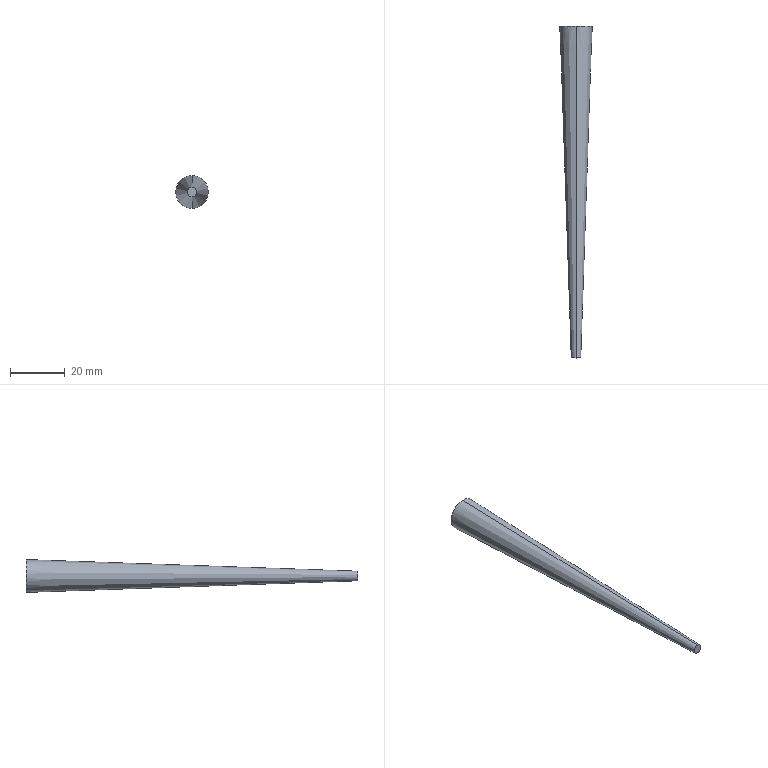Part | STEP file | 1 solid | 4 faces | box 12.021 x 121.757 x 12.021 mm | volume 6349 mm3 | cone 2 | plane 2
STEP:
#1=CARTESIAN_POINT('',(0.,0.,0.));
#2=DIRECTION('',(0.,0.,1.));
#3=DIRECTION('',(1.,0.,0.));
#4=AXIS2_PLACEMENT_3D('',#1,#2,#3);
#5=CARTESIAN_POINT('',(-137.183,8.743,9.799));
#6=VERTEX_POINT('',#5);
#7=CARTESIAN_POINT('',(-137.183,8.743,13.316));
#8=VERTEX_POINT('',#7);
#9=CARTESIAN_POINT('',(-137.183,8.743,11.557));
#10=DIRECTION('',(0.,1.,0.));
#11=DIRECTION('',(0.,0.,-1.));
#12=AXIS2_PLACEMENT_3D('',#9,#10,#11);
#13=CIRCLE('',#12,1.759);
#14=CARTESIAN_POINT('',(-137.183,8.743,11.557));
#15=DIRECTION('',(0.,1.,0.));
#16=DIRECTION('',(0.,0.,-1.));
#17=AXIS2_PLACEMENT_3D('',#14,#15,#16);
#18=CONICAL_SURFACE('',#17,1.759,0.03491);
#19=CARTESIAN_POINT('',(0.,0.));
#20=DIRECTION('',(1.,0.));
#21=VECTOR('',#20,1.);
#22=LINE('',#19,#21);
#23=(GEOMETRIC_REPRESENTATION_CONTEXT(2)PARAMETRIC_REPRESENTATION_CONTEXT()REPRESENTATION_CONTEXT('',''));
#24=DEFINITIONAL_REPRESENTATION('',(#22),#23);
#25=PCURVE('',#18,#24);
#26=CARTESIAN_POINT('',(-137.183,8.743,8.797));
#27=DIRECTION('',(0.,-1.,0.));
#28=DIRECTION('',(0.,0.,-1.));
#29=AXIS2_PLACEMENT_3D('',#26,#27,#28);
#30=PLANE('',#29);
#31=CARTESIAN_POINT('',(-1.001,0.));
#32=CARTESIAN_POINT('',(-1.001,-3.046));
#33=CARTESIAN_POINT('',(-3.64,-1.523));
#34=CARTESIAN_POINT('',(-6.278,0.));
#35=CARTESIAN_POINT('',(-3.64,1.523));
#36=CARTESIAN_POINT('',(-1.001,3.046));
#37=CARTESIAN_POINT('',(-1.001,0.));
#38=(BOUNDED_CURVE()B_SPLINE_CURVE(2,(#31,#32,#33,#34,#35,#36,#37),.UNSPECIFIED.,.T.,.F.)B_SPLINE_CURVE_WITH_KNOTS((1,2,2,2,2,1),(-2.094,0.,2.094,4.189,6.283,8.378),.UNSPECIFIED.)CURVE()GEOMETRIC_REPRESENTATION_ITEM()RATIONAL_B_SPLINE_CURVE((1.,0.5,1.,0.5,1.,0.5,1.))REPRESENTATION_ITEM(''));
#39=(GEOMETRIC_REPRESENTATION_CONTEXT(2)PARAMETRIC_REPRESENTATION_CONTEXT()REPRESENTATION_CONTEXT('',''));
#40=DEFINITIONAL_REPRESENTATION('',(#38),#39);
#41=PCURVE('',#30,#40);
#42=SURFACE_CURVE('',#13,(#25,#41),.PCURVE_S1.);
#43=EDGE_CURVE('',#6,#8,#42,.T.);
#44=ORIENTED_EDGE('',*,*,#43,.T.);
#45=CARTESIAN_POINT('',(-137.183,130.5,17.568));
#46=VERTEX_POINT('',#45);
#47=CARTESIAN_POINT('',(-137.183,8.743,13.316));
#48=DIRECTION('',(0.,0.9994,0.0349));
#49=VECTOR('',#48,1.);
#50=LINE('',#47,#49);
#51=CARTESIAN_POINT('',(3.142,0.));
#52=DIRECTION('',(0.,1.));
#53=VECTOR('',#52,1.);
#54=LINE('',#51,#53);
#55=(GEOMETRIC_REPRESENTATION_CONTEXT(2)PARAMETRIC_REPRESENTATION_CONTEXT()REPRESENTATION_CONTEXT('',''));
#56=DEFINITIONAL_REPRESENTATION('',(#54),#55);
#57=PCURVE('',#18,#56);
#58=CARTESIAN_POINT('',(-137.183,8.743,11.557));
#59=DIRECTION('',(0.,1.,0.));
#60=DIRECTION('',(0.,0.,-1.));
#61=AXIS2_PLACEMENT_3D('',#58,#59,#60);
#62=CONICAL_SURFACE('',#61,1.759,0.03491);
#63=CARTESIAN_POINT('',(3.142,0.));
#64=DIRECTION('',(0.,1.));
#65=VECTOR('',#64,1.);
#66=LINE('',#63,#65);
#67=(GEOMETRIC_REPRESENTATION_CONTEXT(2)PARAMETRIC_REPRESENTATION_CONTEXT()REPRESENTATION_CONTEXT('',''));
#68=DEFINITIONAL_REPRESENTATION('',(#66),#67);
#69=PCURVE('',#62,#68);
#70=SURFACE_CURVE('',#50,(#57,#69),.PCURVE_S1.);
#71=EDGE_CURVE('',#8,#46,#70,.T.);
#72=ORIENTED_EDGE('',*,*,#71,.T.);
#73=CARTESIAN_POINT('',(-137.183,130.5,5.547));
#74=VERTEX_POINT('',#73);
#75=CARTESIAN_POINT('',(-137.183,130.5,11.557));
#76=DIRECTION('',(0.,-1.,0.));
#77=DIRECTION('',(0.,0.,-1.));
#78=AXIS2_PLACEMENT_3D('',#75,#76,#77);
#79=CIRCLE('',#78,6.011);
#80=CARTESIAN_POINT('',(6.283,121.757));
#81=DIRECTION('',(-1.,0.));
#82=VECTOR('',#81,1.);
#83=LINE('',#80,#82);
#84=(GEOMETRIC_REPRESENTATION_CONTEXT(2)PARAMETRIC_REPRESENTATION_CONTEXT()REPRESENTATION_CONTEXT('',''));
#85=DEFINITIONAL_REPRESENTATION('',(#83),#84);
#86=PCURVE('',#18,#85);
#87=CARTESIAN_POINT('',(-72.862,130.5,110.196));
#88=DIRECTION('',(0.,-1.,0.));
#89=DIRECTION('',(0.,0.,-1.));
#90=AXIS2_PLACEMENT_3D('',#87,#88,#89);
#91=PLANE('',#90);
#92=CARTESIAN_POINT('',(98.638,-64.32));
#93=DIRECTION('',(1.,0.));
#94=AXIS2_PLACEMENT_2D('',#92,#93);
#95=CIRCLE('',#94,6.011);
#96=(GEOMETRIC_REPRESENTATION_CONTEXT(2)PARAMETRIC_REPRESENTATION_CONTEXT()REPRESENTATION_CONTEXT('',''));
#97=DEFINITIONAL_REPRESENTATION('',(#95),#96);
#98=PCURVE('',#91,#97);
#99=SURFACE_CURVE('',#79,(#86,#98),.PCURVE_S1.);
#100=EDGE_CURVE('',#46,#74,#99,.T.);
#101=ORIENTED_EDGE('',*,*,#100,.T.);
#102=CARTESIAN_POINT('',(-137.183,8.743,9.799));
#103=DIRECTION('',(0.,0.9994,-0.0349));
#104=VECTOR('',#103,1.);
#105=LINE('',#102,#104);
#106=CARTESIAN_POINT('',(0.,0.));
#107=DIRECTION('',(0.,1.));
#108=VECTOR('',#107,1.);
#109=LINE('',#106,#108);
#110=(GEOMETRIC_REPRESENTATION_CONTEXT(2)PARAMETRIC_REPRESENTATION_CONTEXT()REPRESENTATION_CONTEXT('',''));
#111=DEFINITIONAL_REPRESENTATION('',(#109),#110);
#112=PCURVE('',#18,#111);
#113=CARTESIAN_POINT('',(6.283,0.));
#114=DIRECTION('',(0.,1.));
#115=VECTOR('',#114,1.);
#116=LINE('',#113,#115);
#117=(GEOMETRIC_REPRESENTATION_CONTEXT(2)PARAMETRIC_REPRESENTATION_CONTEXT()REPRESENTATION_CONTEXT('',''));
#118=DEFINITIONAL_REPRESENTATION('',(#116),#117);
#119=PCURVE('',#62,#118);
#120=SURFACE_CURVE('',#105,(#112,#119),.PCURVE_S1.);
#121=EDGE_CURVE('',#6,#74,#120,.T.);
#122=ORIENTED_EDGE('',*,*,#121,.F.);
#123=EDGE_LOOP('',(#44,#72,#101,#122));
#124=FACE_BOUND('',#123,.T.);
#125=ADVANCED_FACE('',(#124),#18,.T.);
#126=ORIENTED_EDGE('',*,*,#71,.F.);
#127=CARTESIAN_POINT('',(-137.183,8.743,11.557));
#128=DIRECTION('',(0.,1.,0.));
#129=DIRECTION('',(0.,0.,-1.));
#130=AXIS2_PLACEMENT_3D('',#127,#128,#129);
#131=CIRCLE('',#130,1.759);
#132=CARTESIAN_POINT('',(0.,0.));
#133=DIRECTION('',(1.,0.));
#134=VECTOR('',#133,1.);
#135=LINE('',#132,#134);
#136=(GEOMETRIC_REPRESENTATION_CONTEXT(2)PARAMETRIC_REPRESENTATION_CONTEXT()REPRESENTATION_CONTEXT('',''));
#137=DEFINITIONAL_REPRESENTATION('',(#135),#136);
#138=PCURVE('',#62,#137);
#139=CARTESIAN_POINT('',(-1.001,0.));
#140=CARTESIAN_POINT('',(-1.001,-3.046));
#141=CARTESIAN_POINT('',(-3.64,-1.523));
#142=CARTESIAN_POINT('',(-6.278,0.));
#143=CARTESIAN_POINT('',(-3.64,1.523));
#144=CARTESIAN_POINT('',(-1.001,3.046));
#145=CARTESIAN_POINT('',(-1.001,0.));
#146=(BOUNDED_CURVE()B_SPLINE_CURVE(2,(#139,#140,#141,#142,#143,#144,#145),.UNSPECIFIED.,.T.,.F.)B_SPLINE_CURVE_WITH_KNOTS((1,2,2,2,2,1),(-2.094,0.,2.094,4.189,6.283,8.378),.UNSPECIFIED.)CURVE()GEOMETRIC_REPRESENTATION_ITEM()RATIONAL_B_SPLINE_CURVE((1.,0.5,1.,0.5,1.,0.5,1.))REPRESENTATION_ITEM(''));
#147=(GEOMETRIC_REPRESENTATION_CONTEXT(2)PARAMETRIC_REPRESENTATION_CONTEXT()REPRESENTATION_CONTEXT('',''));
#148=DEFINITIONAL_REPRESENTATION('',(#146),#147);
#149=PCURVE('',#30,#148);
#150=SURFACE_CURVE('',#131,(#138,#149),.PCURVE_S1.);
#151=EDGE_CURVE('',#8,#6,#150,.T.);
#152=ORIENTED_EDGE('',*,*,#151,.T.);
#153=ORIENTED_EDGE('',*,*,#121,.T.);
#154=CARTESIAN_POINT('',(-137.183,130.5,11.557));
#155=DIRECTION('',(0.,-1.,0.));
#156=DIRECTION('',(0.,0.,-1.));
#157=AXIS2_PLACEMENT_3D('',#154,#155,#156);
#158=CIRCLE('',#157,6.011);
#159=CARTESIAN_POINT('',(6.283,121.757));
#160=DIRECTION('',(-1.,0.));
#161=VECTOR('',#160,1.);
#162=LINE('',#159,#161);
#163=(GEOMETRIC_REPRESENTATION_CONTEXT(2)PARAMETRIC_REPRESENTATION_CONTEXT()REPRESENTATION_CONTEXT('',''));
#164=DEFINITIONAL_REPRESENTATION('',(#162),#163);
#165=PCURVE('',#62,#164);
#166=CARTESIAN_POINT('',(98.638,-64.32));
#167=DIRECTION('',(1.,0.));
#168=AXIS2_PLACEMENT_2D('',#166,#167);
#169=CIRCLE('',#168,6.011);
#170=(GEOMETRIC_REPRESENTATION_CONTEXT(2)PARAMETRIC_REPRESENTATION_CONTEXT()REPRESENTATION_CONTEXT('',''));
#171=DEFINITIONAL_REPRESENTATION('',(#169),#170);
#172=PCURVE('',#91,#171);
#173=SURFACE_CURVE('',#158,(#165,#172),.PCURVE_S1.);
#174=EDGE_CURVE('',#74,#46,#173,.T.);
#175=ORIENTED_EDGE('',*,*,#174,.T.);
#176=EDGE_LOOP('',(#126,#152,#153,#175));
#177=FACE_BOUND('',#176,.T.);
#178=ADVANCED_FACE('',(#177),#62,.T.);
#179=ORIENTED_EDGE('',*,*,#43,.F.);
#180=ORIENTED_EDGE('',*,*,#151,.F.);
#181=EDGE_LOOP('',(#179,#180));
#182=FACE_BOUND('',#181,.T.);
#183=ADVANCED_FACE('',(#182),#30,.T.);
#184=ORIENTED_EDGE('',*,*,#174,.F.);
#185=ORIENTED_EDGE('',*,*,#100,.F.);
#186=EDGE_LOOP('',(#184,#185));
#187=FACE_BOUND('',#186,.T.);
#188=ADVANCED_FACE('',(#187),#91,.F.);
#189=CLOSED_SHELL('',(#125,#178,#183,#188));
#190=MANIFOLD_SOLID_BREP('',#189);
#191=(LENGTH_UNIT()NAMED_UNIT(*)SI_UNIT(.MILLI.,.METRE.));
#192=UNCERTAINTY_MEASURE_WITH_UNIT(LENGTH_MEASURE(0.0000001),#191,'','');
#193=(NAMED_UNIT(*)PLANE_ANGLE_UNIT()SI_UNIT($,.RADIAN.));
#194=(NAMED_UNIT(*)SI_UNIT($,.STERADIAN.)SOLID_ANGLE_UNIT());
#195=(GEOMETRIC_REPRESENTATION_CONTEXT(3)GLOBAL_UNCERTAINTY_ASSIGNED_CONTEXT((#192))GLOBAL_UNIT_ASSIGNED_CONTEXT((#191,#193,#194))REPRESENTATION_CONTEXT('',''));
#196=ADVANCED_BREP_SHAPE_REPRESENTATION('',(#4,#190),#195);